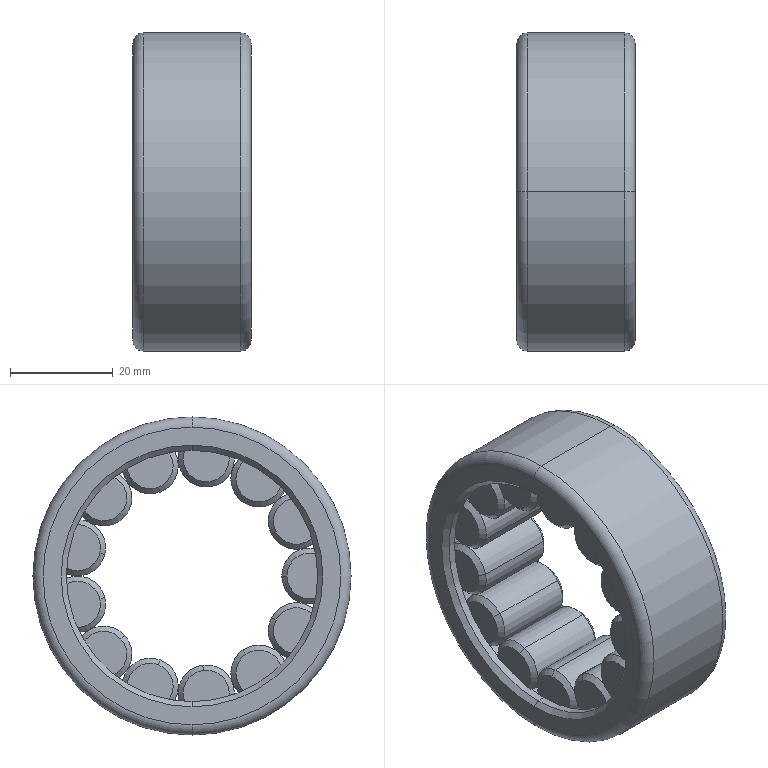Part | SolidWorks | features BaseBody 1 | 1 solid | 293 faces | box 23 x 62 x 62 mm | volume 35184 mm3 | spline 106 | plane 89 | cone 56 | cylinder 34 | torus 8 | commonest cylinder face diameters 10.97 x26 49 x4 57 x2 62 x2